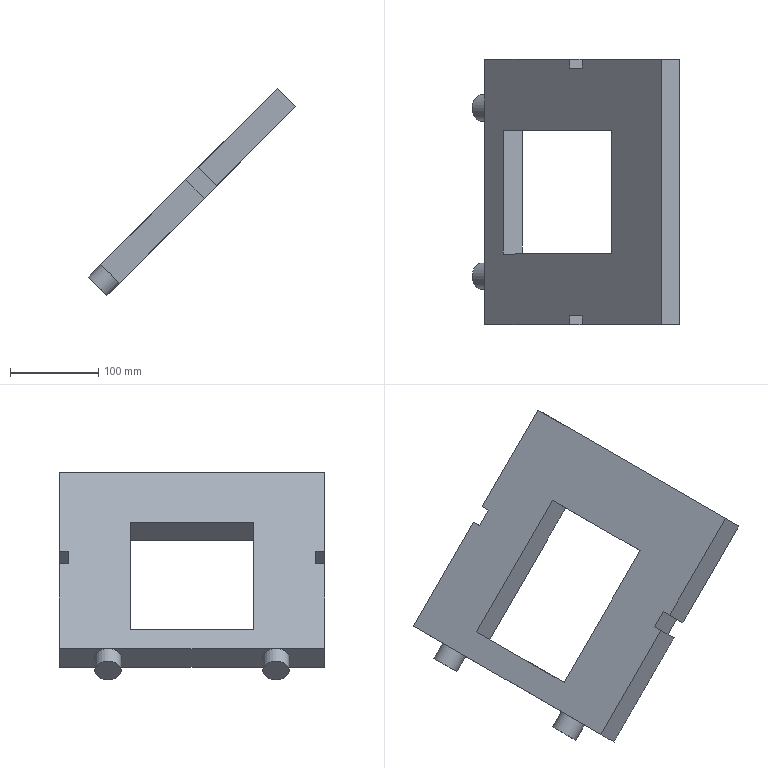Part | NX | features solid 2 | 1 solid | 24 faces | box 234.759 x 300 x 234.759 mm | volume 1831955 mm3 | plane 22 | cylinder 2 | commonest cylinder face diameters 30 x2
STEP:
#1=CARTESIAN_POINT('',(-1080.504,275.,-210.197));
#2=VERTEX_POINT('',#1);
#3=CARTESIAN_POINT('',(-1101.717,275.,-188.984));
#4=VERTEX_POINT('',#3);
#5=CARTESIAN_POINT('',(-1091.111,275.,-199.591));
#6=DIRECTION('',(-0.7071,0.,-0.7071));
#7=DIRECTION('',(0.7071,0.,-0.7071));
#8=AXIS2_PLACEMENT_3D('',#5,#6,#7);
#9=CIRCLE('',#8,15.);
#10=EDGE_CURVE('',#2,#4,#9,.T.);
#11=ORIENTED_EDGE('',*,*,#10,.F.);
#12=CARTESIAN_POINT('',(-1080.504,85.,-210.197));
#13=VERTEX_POINT('',#12);
#14=CARTESIAN_POINT('',(-1080.504,30.,-210.197));
#15=DIRECTION('',(0.,1.,0.));
#16=VECTOR('',#15,1000.);
#17=LINE('',#14,#16);
#18=EDGE_CURVE('',#13,#2,#17,.T.);
#19=ORIENTED_EDGE('',*,*,#18,.F.);
#20=CARTESIAN_POINT('',(-1101.717,85.,-188.984));
#21=VERTEX_POINT('',#20);
#22=CARTESIAN_POINT('',(-1091.111,85.,-199.591));
#23=DIRECTION('',(-0.7071,0.,-0.7071));
#24=DIRECTION('',(0.7071,0.,-0.7071));
#25=AXIS2_PLACEMENT_3D('',#22,#23,#24);
#26=CIRCLE('',#25,15.);
#27=EDGE_CURVE('',#21,#13,#26,.T.);
#28=ORIENTED_EDGE('',*,*,#27,.F.);
#29=CARTESIAN_POINT('',(-1101.717,30.,-188.984));
#30=DIRECTION('',(0.,1.,0.));
#31=VECTOR('',#30,1000.);
#32=LINE('',#29,#31);
#33=EDGE_CURVE('',#21,#4,#32,.T.);
#34=ORIENTED_EDGE('',*,*,#33,.T.);
#35=EDGE_LOOP('',(#11,#19,#28,#34));
#36=FACE_BOUND('',#35,.T.);
#37=CARTESIAN_POINT('',(-1080.504,30.,-210.197));
#38=DIRECTION('',(-0.7071,0.,-0.7071));
#39=DIRECTION('',(0.7071,0.,-0.7071));
#40=AXIS2_PLACEMENT_3D('',#37,#38,#39);
#41=PLANE('',#40);
#42=ADVANCED_FACE('',(#36),#41,.T.);
#43=CARTESIAN_POINT('',(-1091.111,85.,-199.591));
#44=DIRECTION('',(-0.7071,0.,-0.7071));
#45=DIRECTION('',(0.7071,0.,-0.7071));
#46=AXIS2_PLACEMENT_3D('',#43,#44,#45);
#47=CIRCLE('',#46,15.);
#48=EDGE_CURVE('',#13,#21,#47,.T.);
#49=ORIENTED_EDGE('',*,*,#48,.F.);
#50=CARTESIAN_POINT('',(-1080.504,30.,-210.197));
#51=VERTEX_POINT('',#50);
#52=CARTESIAN_POINT('',(-1080.504,30.,-210.197));
#53=DIRECTION('',(0.,1.,0.));
#54=VECTOR('',#53,1000.);
#55=LINE('',#52,#54);
#56=EDGE_CURVE('',#51,#13,#55,.T.);
#57=ORIENTED_EDGE('',*,*,#56,.F.);
#58=CARTESIAN_POINT('',(-1101.717,30.,-188.984));
#59=VERTEX_POINT('',#58);
#60=CARTESIAN_POINT('',(-1080.504,30.,-210.197));
#61=DIRECTION('',(-0.7071,0.,0.7071));
#62=VECTOR('',#61,1000.);
#63=LINE('',#60,#62);
#64=EDGE_CURVE('',#51,#59,#63,.T.);
#65=ORIENTED_EDGE('',*,*,#64,.T.);
#66=CARTESIAN_POINT('',(-1101.717,30.,-188.984));
#67=DIRECTION('',(0.,1.,0.));
#68=VECTOR('',#67,1000.);
#69=LINE('',#66,#68);
#70=EDGE_CURVE('',#59,#21,#69,.T.);
#71=ORIENTED_EDGE('',*,*,#70,.T.);
#72=EDGE_LOOP('',(#49,#57,#65,#71));
#73=FACE_BOUND('',#72,.T.);
#74=CARTESIAN_POINT('',(-1080.504,30.,-210.197));
#75=DIRECTION('',(-0.7071,0.,-0.7071));
#76=DIRECTION('',(0.7071,0.,-0.7071));
#77=AXIS2_PLACEMENT_3D('',#74,#75,#76);
#78=PLANE('',#77);
#79=ADVANCED_FACE('',(#73),#78,.T.);
#80=CARTESIAN_POINT('',(-991.665,30.,-78.932));
#81=VERTEX_POINT('',#80);
#82=CARTESIAN_POINT('',(-902.313,30.,10.42));
#83=VERTEX_POINT('',#82);
#84=CARTESIAN_POINT('',(-1137.073,30.,-224.34));
#85=DIRECTION('',(0.7071,0.,0.7071));
#86=VECTOR('',#85,1000.);
#87=LINE('',#84,#86);
#88=EDGE_CURVE('',#81,#83,#87,.T.);
#89=ORIENTED_EDGE('',*,*,#88,.F.);
#90=CARTESIAN_POINT('',(-970.452,30.,-100.145));
#91=VERTEX_POINT('',#90);
#92=CARTESIAN_POINT('',(-1023.864,30.,-46.733));
#93=DIRECTION('',(-0.7071,0.,0.7071));
#94=VECTOR('',#93,1000.);
#95=LINE('',#92,#94);
#96=EDGE_CURVE('',#91,#81,#95,.T.);
#97=ORIENTED_EDGE('',*,*,#96,.F.);
#98=CARTESIAN_POINT('',(-881.1,30.,-10.793));
#99=VERTEX_POINT('',#98);
#100=CARTESIAN_POINT('',(-916.455,30.,-46.149));
#101=DIRECTION('',(-0.7071,0.,-0.7071));
#102=VECTOR('',#101,1000.);
#103=LINE('',#100,#102);
#104=EDGE_CURVE('',#99,#91,#103,.T.);
#105=ORIENTED_EDGE('',*,*,#104,.F.);
#106=CARTESIAN_POINT('',(-902.313,30.,10.42));
#107=DIRECTION('',(0.7071,0.,-0.7071));
#108=VECTOR('',#107,1000.);
#109=LINE('',#106,#108);
#110=EDGE_CURVE('',#83,#99,#109,.T.);
#111=ORIENTED_EDGE('',*,*,#110,.F.);
#112=EDGE_LOOP('',(#89,#97,#105,#111));
#113=FACE_BOUND('',#112,.T.);
#114=CARTESIAN_POINT('',(-1137.073,30.,-224.34));
#115=DIRECTION('',(0.,-1.,0.));
#116=DIRECTION('',(0.9963,0.,0.08598));
#117=AXIS2_PLACEMENT_3D('',#114,#115,#116);
#118=PLANE('',#117);
#119=ADVANCED_FACE('',(#113),#118,.T.);
#120=CARTESIAN_POINT('',(-958.882,250.,-46.149));
#121=VERTEX_POINT('',#120);
#122=CARTESIAN_POINT('',(-958.882,110.,-46.149));
#123=VERTEX_POINT('',#122);
#124=CARTESIAN_POINT('',(-958.882,250.,-46.149));
#125=DIRECTION('',(0.,-1.,0.));
#126=VECTOR('',#125,1000.);
#127=LINE('',#124,#126);
#128=EDGE_CURVE('',#121,#123,#127,.T.);
#129=ORIENTED_EDGE('',*,*,#128,.T.);
#130=CARTESIAN_POINT('',(-1080.504,110.,-167.771));
#131=VERTEX_POINT('',#130);
#132=CARTESIAN_POINT('',(-1137.073,110.,-224.34));
#133=DIRECTION('',(0.7071,0.,0.7071));
#134=VECTOR('',#133,1000.);
#135=LINE('',#132,#134);
#136=EDGE_CURVE('',#131,#123,#135,.T.);
#137=ORIENTED_EDGE('',*,*,#136,.F.);
#138=CARTESIAN_POINT('',(-1080.504,250.,-167.771));
#139=VERTEX_POINT('',#138);
#140=CARTESIAN_POINT('',(-1080.504,250.,-167.771));
#141=DIRECTION('',(0.,-1.,0.));
#142=VECTOR('',#141,1000.);
#143=LINE('',#140,#142);
#144=EDGE_CURVE('',#139,#131,#143,.T.);
#145=ORIENTED_EDGE('',*,*,#144,.F.);
#146=CARTESIAN_POINT('',(-1137.073,250.,-224.34));
#147=DIRECTION('',(0.7071,0.,0.7071));
#148=VECTOR('',#147,1000.);
#149=LINE('',#146,#148);
#150=EDGE_CURVE('',#139,#121,#149,.T.);
#151=ORIENTED_EDGE('',*,*,#150,.T.);
#152=EDGE_LOOP('',(#129,#137,#145,#151));
#153=FACE_BOUND('',#152,.T.);
#154=CARTESIAN_POINT('',(-1005.712,30.,-92.979));
#155=VERTEX_POINT('',#154);
#156=CARTESIAN_POINT('',(-1005.712,40.,-92.979));
#157=VERTEX_POINT('',#156);
#158=CARTESIAN_POINT('',(-1005.712,40.,-92.979));
#159=DIRECTION('',(0.,1.,0.));
#160=VECTOR('',#159,1000.);
#161=LINE('',#158,#160);
#162=EDGE_CURVE('',#155,#157,#161,.T.);
#163=ORIENTED_EDGE('',*,*,#162,.T.);
#164=CARTESIAN_POINT('',(-991.665,40.,-78.932));
#165=VERTEX_POINT('',#164);
#166=CARTESIAN_POINT('',(-1137.073,40.,-224.34));
#167=DIRECTION('',(0.7071,0.,0.7071));
#168=VECTOR('',#167,1000.);
#169=LINE('',#166,#168);
#170=EDGE_CURVE('',#165,#157,#169,.F.);
#171=ORIENTED_EDGE('',*,*,#170,.F.);
#172=CARTESIAN_POINT('',(-991.665,40.,-78.932));
#173=DIRECTION('',(0.,1.,0.));
#174=VECTOR('',#173,1000.);
#175=LINE('',#172,#174);
#176=EDGE_CURVE('',#81,#165,#175,.T.);
#177=ORIENTED_EDGE('',*,*,#176,.F.);
#178=ORIENTED_EDGE('',*,*,#88,.T.);
#179=CARTESIAN_POINT('',(-902.313,330.,10.42));
#180=VERTEX_POINT('',#179);
#181=CARTESIAN_POINT('',(-902.313,30.,10.42));
#182=DIRECTION('',(0.,1.,0.));
#183=VECTOR('',#182,1000.);
#184=LINE('',#181,#183);
#185=EDGE_CURVE('',#83,#180,#184,.T.);
#186=ORIENTED_EDGE('',*,*,#185,.T.);
#187=CARTESIAN_POINT('',(-991.665,330.,-78.932));
#188=VERTEX_POINT('',#187);
#189=CARTESIAN_POINT('',(-1137.073,330.,-224.34));
#190=DIRECTION('',(0.7071,0.,0.7071));
#191=VECTOR('',#190,1000.);
#192=LINE('',#189,#191);
#193=EDGE_CURVE('',#188,#180,#192,.T.);
#194=ORIENTED_EDGE('',*,*,#193,.F.);
#195=CARTESIAN_POINT('',(-991.665,320.,-78.932));
#196=VERTEX_POINT('',#195);
#197=CARTESIAN_POINT('',(-991.665,320.,-78.932));
#198=DIRECTION('',(0.,1.,0.));
#199=VECTOR('',#198,1000.);
#200=LINE('',#197,#199);
#201=EDGE_CURVE('',#188,#196,#200,.F.);
#202=ORIENTED_EDGE('',*,*,#201,.T.);
#203=CARTESIAN_POINT('',(-1005.712,320.,-92.979));
#204=VERTEX_POINT('',#203);
#205=CARTESIAN_POINT('',(-1137.073,320.,-224.34));
#206=DIRECTION('',(0.7071,0.,0.7071));
#207=VECTOR('',#206,1000.);
#208=LINE('',#205,#207);
#209=EDGE_CURVE('',#196,#204,#208,.F.);
#210=ORIENTED_EDGE('',*,*,#209,.T.);
#211=CARTESIAN_POINT('',(-1005.712,330.,-92.979));
#212=VERTEX_POINT('',#211);
#213=CARTESIAN_POINT('',(-1005.712,320.,-92.979));
#214=DIRECTION('',(0.,1.,0.));
#215=VECTOR('',#214,1000.);
#216=LINE('',#213,#215);
#217=EDGE_CURVE('',#212,#204,#216,.F.);
#218=ORIENTED_EDGE('',*,*,#217,.F.);
#219=CARTESIAN_POINT('',(-1101.717,330.,-188.984));
#220=VERTEX_POINT('',#219);
#221=CARTESIAN_POINT('',(-1137.073,330.,-224.34));
#222=DIRECTION('',(0.7071,0.,0.7071));
#223=VECTOR('',#222,1000.);
#224=LINE('',#221,#223);
#225=EDGE_CURVE('',#220,#212,#224,.T.);
#226=ORIENTED_EDGE('',*,*,#225,.F.);
#227=CARTESIAN_POINT('',(-1101.717,30.,-188.984));
#228=DIRECTION('',(0.,1.,0.));
#229=VECTOR('',#228,1000.);
#230=LINE('',#227,#229);
#231=EDGE_CURVE('',#4,#220,#230,.T.);
#232=ORIENTED_EDGE('',*,*,#231,.F.);
#233=ORIENTED_EDGE('',*,*,#33,.F.);
#234=ORIENTED_EDGE('',*,*,#70,.F.);
#235=CARTESIAN_POINT('',(-1137.073,30.,-224.34));
#236=DIRECTION('',(0.7071,0.,0.7071));
#237=VECTOR('',#236,1000.);
#238=LINE('',#235,#237);
#239=EDGE_CURVE('',#59,#155,#238,.T.);
#240=ORIENTED_EDGE('',*,*,#239,.T.);
#241=EDGE_LOOP('',(#163,#171,#177,#178,#186,#194,#202,#210,#218,#226,#232,#233,#234,#240));
#242=FACE_BOUND('',#241,.T.);
#243=CARTESIAN_POINT('',(-1137.073,30.,-224.34));
#244=DIRECTION('',(-0.7071,0.,0.7071));
#245=DIRECTION('',(-0.7071,0.,-0.7071));
#246=AXIS2_PLACEMENT_3D('',#243,#244,#245);
#247=PLANE('',#246);
#248=ADVANCED_FACE('',(#153,#242),#247,.T.);
#249=CARTESIAN_POINT('',(-881.1,330.,-10.793));
#250=VERTEX_POINT('',#249);
#251=CARTESIAN_POINT('',(-881.1,30.,-10.793));
#252=DIRECTION('',(0.,1.,0.));
#253=VECTOR('',#252,1000.);
#254=LINE('',#251,#253);
#255=EDGE_CURVE('',#99,#250,#254,.T.);
#256=ORIENTED_EDGE('',*,*,#255,.T.);
#257=CARTESIAN_POINT('',(-902.313,330.,10.42));
#258=DIRECTION('',(0.7071,0.,-0.7071));
#259=VECTOR('',#258,1000.);
#260=LINE('',#257,#259);
#261=EDGE_CURVE('',#180,#250,#260,.T.);
#262=ORIENTED_EDGE('',*,*,#261,.F.);
#263=ORIENTED_EDGE('',*,*,#185,.F.);
#264=ORIENTED_EDGE('',*,*,#110,.T.);
#265=EDGE_LOOP('',(#256,#262,#263,#264));
#266=FACE_BOUND('',#265,.T.);
#267=CARTESIAN_POINT('',(-902.313,30.,10.42));
#268=DIRECTION('',(0.7071,0.,0.7071));
#269=DIRECTION('',(-0.7071,0.,0.7071));
#270=AXIS2_PLACEMENT_3D('',#267,#268,#269);
#271=PLANE('',#270);
#272=ADVANCED_FACE('',(#266),#271,.T.);
#273=CARTESIAN_POINT('',(-1059.291,250.,-188.984));
#274=VERTEX_POINT('',#273);
#275=CARTESIAN_POINT('',(-1059.291,110.,-188.984));
#276=VERTEX_POINT('',#275);
#277=CARTESIAN_POINT('',(-1059.291,250.,-188.984));
#278=DIRECTION('',(0.,-1.,0.));
#279=VECTOR('',#278,1000.);
#280=LINE('',#277,#279);
#281=EDGE_CURVE('',#274,#276,#280,.T.);
#282=ORIENTED_EDGE('',*,*,#281,.T.);
#283=CARTESIAN_POINT('',(-937.669,110.,-67.362));
#284=VERTEX_POINT('',#283);
#285=CARTESIAN_POINT('',(-916.455,110.,-46.149));
#286=DIRECTION('',(-0.7071,0.,-0.7071));
#287=VECTOR('',#286,1000.);
#288=LINE('',#285,#287);
#289=EDGE_CURVE('',#284,#276,#288,.T.);
#290=ORIENTED_EDGE('',*,*,#289,.F.);
#291=CARTESIAN_POINT('',(-937.669,250.,-67.362));
#292=VERTEX_POINT('',#291);
#293=CARTESIAN_POINT('',(-937.669,250.,-67.362));
#294=DIRECTION('',(0.,-1.,0.));
#295=VECTOR('',#294,1000.);
#296=LINE('',#293,#295);
#297=EDGE_CURVE('',#292,#284,#296,.T.);
#298=ORIENTED_EDGE('',*,*,#297,.F.);
#299=CARTESIAN_POINT('',(-916.455,250.,-46.149));
#300=DIRECTION('',(-0.7071,0.,-0.7071));
#301=VECTOR('',#300,1000.);
#302=LINE('',#299,#301);
#303=EDGE_CURVE('',#292,#274,#302,.T.);
#304=ORIENTED_EDGE('',*,*,#303,.T.);
#305=EDGE_LOOP('',(#282,#290,#298,#304));
#306=FACE_BOUND('',#305,.T.);
#307=CARTESIAN_POINT('',(-984.499,30.,-114.192));
#308=VERTEX_POINT('',#307);
#309=CARTESIAN_POINT('',(-984.499,40.,-114.192));
#310=VERTEX_POINT('',#309);
#311=CARTESIAN_POINT('',(-984.499,30.,-114.192));
#312=DIRECTION('',(0.,1.,0.));
#313=VECTOR('',#312,1000.);
#314=LINE('',#311,#313);
#315=EDGE_CURVE('',#308,#310,#314,.T.);
#316=ORIENTED_EDGE('',*,*,#315,.F.);
#317=CARTESIAN_POINT('',(-916.455,30.,-46.149));
#318=DIRECTION('',(-0.7071,0.,-0.7071));
#319=VECTOR('',#318,1000.);
#320=LINE('',#317,#319);
#321=EDGE_CURVE('',#308,#51,#320,.T.);
#322=ORIENTED_EDGE('',*,*,#321,.T.);
#323=ORIENTED_EDGE('',*,*,#56,.T.);
#324=ORIENTED_EDGE('',*,*,#18,.T.);
#325=CARTESIAN_POINT('',(-1080.504,330.,-210.197));
#326=VERTEX_POINT('',#325);
#327=CARTESIAN_POINT('',(-1080.504,30.,-210.197));
#328=DIRECTION('',(0.,1.,0.));
#329=VECTOR('',#328,1000.);
#330=LINE('',#327,#329);
#331=EDGE_CURVE('',#2,#326,#330,.T.);
#332=ORIENTED_EDGE('',*,*,#331,.T.);
#333=CARTESIAN_POINT('',(-984.499,330.,-114.192));
#334=VERTEX_POINT('',#333);
#335=CARTESIAN_POINT('',(-916.455,330.,-46.149));
#336=DIRECTION('',(-0.7071,0.,-0.7071));
#337=VECTOR('',#336,1000.);
#338=LINE('',#335,#337);
#339=EDGE_CURVE('',#334,#326,#338,.T.);
#340=ORIENTED_EDGE('',*,*,#339,.F.);
#341=CARTESIAN_POINT('',(-984.499,320.,-114.192));
#342=VERTEX_POINT('',#341);
#343=CARTESIAN_POINT('',(-984.499,30.,-114.192));
#344=DIRECTION('',(0.,1.,0.));
#345=VECTOR('',#344,1000.);
#346=LINE('',#343,#345);
#347=EDGE_CURVE('',#334,#342,#346,.F.);
#348=ORIENTED_EDGE('',*,*,#347,.T.);
#349=CARTESIAN_POINT('',(-970.452,320.,-100.145));
#350=VERTEX_POINT('',#349);
#351=CARTESIAN_POINT('',(-1115.86,320.,-245.553));
#352=DIRECTION('',(0.7071,0.,0.7071));
#353=VECTOR('',#352,1000.);
#354=LINE('',#351,#353);
#355=EDGE_CURVE('',#350,#342,#354,.F.);
#356=ORIENTED_EDGE('',*,*,#355,.F.);
#357=CARTESIAN_POINT('',(-970.452,330.,-100.145));
#358=VERTEX_POINT('',#357);
#359=CARTESIAN_POINT('',(-970.452,30.,-100.145));
#360=DIRECTION('',(0.,1.,0.));
#361=VECTOR('',#360,1000.);
#362=LINE('',#359,#361);
#363=EDGE_CURVE('',#358,#350,#362,.F.);
#364=ORIENTED_EDGE('',*,*,#363,.F.);
#365=CARTESIAN_POINT('',(-916.455,330.,-46.149));
#366=DIRECTION('',(-0.7071,0.,-0.7071));
#367=VECTOR('',#366,1000.);
#368=LINE('',#365,#367);
#369=EDGE_CURVE('',#250,#358,#368,.T.);
#370=ORIENTED_EDGE('',*,*,#369,.F.);
#371=ORIENTED_EDGE('',*,*,#255,.F.);
#372=ORIENTED_EDGE('',*,*,#104,.T.);
#373=CARTESIAN_POINT('',(-970.452,40.,-100.145));
#374=VERTEX_POINT('',#373);
#375=CARTESIAN_POINT('',(-970.452,30.,-100.145));
#376=DIRECTION('',(0.,1.,0.));
#377=VECTOR('',#376,1000.);
#378=LINE('',#375,#377);
#379=EDGE_CURVE('',#91,#374,#378,.T.);
#380=ORIENTED_EDGE('',*,*,#379,.T.);
#381=CARTESIAN_POINT('',(-1115.86,40.,-245.553));
#382=DIRECTION('',(0.7071,0.,0.7071));
#383=VECTOR('',#382,1000.);
#384=LINE('',#381,#383);
#385=EDGE_CURVE('',#374,#310,#384,.F.);
#386=ORIENTED_EDGE('',*,*,#385,.T.);
#387=EDGE_LOOP('',(#316,#322,#323,#324,#332,#340,#348,#356,#364,#370,#371,#372,#380,#386));
#388=FACE_BOUND('',#387,.T.);
#389=CARTESIAN_POINT('',(-916.455,30.,-46.149));
#390=DIRECTION('',(0.7071,0.,-0.7071));
#391=DIRECTION('',(0.7071,0.,0.7071));
#392=AXIS2_PLACEMENT_3D('',#389,#390,#391);
#393=PLANE('',#392);
#394=ADVANCED_FACE('',(#306,#388),#393,.T.);
#395=CARTESIAN_POINT('',(-1091.111,275.,-199.591));
#396=DIRECTION('',(0.7071,0.,0.7071));
#397=DIRECTION('',(0.7071,0.,-0.7071));
#398=AXIS2_PLACEMENT_3D('',#395,#396,#397);
#399=CIRCLE('',#398,15.);
#400=EDGE_CURVE('',#2,#4,#399,.T.);
#401=ORIENTED_EDGE('',*,*,#400,.T.);
#402=ORIENTED_EDGE('',*,*,#231,.T.);
#403=CARTESIAN_POINT('',(-1080.504,330.,-210.197));
#404=DIRECTION('',(-0.7071,0.,0.7071));
#405=VECTOR('',#404,1000.);
#406=LINE('',#403,#405);
#407=EDGE_CURVE('',#326,#220,#406,.T.);
#408=ORIENTED_EDGE('',*,*,#407,.F.);
#409=ORIENTED_EDGE('',*,*,#331,.F.);
#410=EDGE_LOOP('',(#401,#402,#408,#409));
#411=FACE_BOUND('',#410,.T.);
#412=CARTESIAN_POINT('',(-1080.504,30.,-210.197));
#413=DIRECTION('',(-0.7071,0.,-0.7071));
#414=DIRECTION('',(0.7071,0.,-0.7071));
#415=AXIS2_PLACEMENT_3D('',#412,#413,#414);
#416=PLANE('',#415);
#417=ADVANCED_FACE('',(#411),#416,.T.);
#418=CARTESIAN_POINT('',(-1036.273,30.,-62.418));
#419=DIRECTION('',(-0.7071,0.,0.7071));
#420=VECTOR('',#419,1000.);
#421=LINE('',#418,#420);
#422=EDGE_CURVE('',#308,#155,#421,.T.);
#423=ORIENTED_EDGE('',*,*,#422,.T.);
#424=ORIENTED_EDGE('',*,*,#239,.F.);
#425=ORIENTED_EDGE('',*,*,#64,.F.);
#426=ORIENTED_EDGE('',*,*,#321,.F.);
#427=EDGE_LOOP('',(#423,#424,#425,#426));
#428=FACE_BOUND('',#427,.T.);
#429=CARTESIAN_POINT('',(-1137.073,30.,-224.34));
#430=DIRECTION('',(0.,-1.,0.));
#431=DIRECTION('',(0.9963,0.,0.08598));
#432=AXIS2_PLACEMENT_3D('',#429,#430,#431);
#433=PLANE('',#432);
#434=ADVANCED_FACE('',(#428),#433,.T.);
#435=ORIENTED_EDGE('',*,*,#289,.T.);
#436=CARTESIAN_POINT('',(-1059.291,110.,-188.984));
#437=DIRECTION('',(-0.7071,0.,0.7071));
#438=VECTOR('',#437,1000.);
#439=LINE('',#436,#438);
#440=EDGE_CURVE('',#276,#131,#439,.T.);
#441=ORIENTED_EDGE('',*,*,#440,.T.);
#442=ORIENTED_EDGE('',*,*,#136,.T.);
#443=CARTESIAN_POINT('',(-958.882,110.,-46.149));
#444=DIRECTION('',(0.7071,0.,-0.7071));
#445=VECTOR('',#444,1000.);
#446=LINE('',#443,#445);
#447=EDGE_CURVE('',#123,#284,#446,.T.);
#448=ORIENTED_EDGE('',*,*,#447,.T.);
#449=EDGE_LOOP('',(#435,#441,#442,#448));
#450=FACE_BOUND('',#449,.T.);
#451=CARTESIAN_POINT('',(-1137.073,110.,-224.34));
#452=DIRECTION('',(0.,-1.,0.));
#453=DIRECTION('',(0.9963,0.,0.08598));
#454=AXIS2_PLACEMENT_3D('',#451,#452,#453);
#455=PLANE('',#454);
#456=ADVANCED_FACE('',(#450),#455,.F.);
#457=ORIENTED_EDGE('',*,*,#385,.F.);
#458=CARTESIAN_POINT('',(-1023.864,40.,-46.733));
#459=DIRECTION('',(-0.7071,0.,0.7071));
#460=VECTOR('',#459,1000.);
#461=LINE('',#458,#460);
#462=EDGE_CURVE('',#374,#165,#461,.T.);
#463=ORIENTED_EDGE('',*,*,#462,.T.);
#464=ORIENTED_EDGE('',*,*,#170,.T.);
#465=CARTESIAN_POINT('',(-1036.273,40.,-62.418));
#466=DIRECTION('',(-0.7071,0.,0.7071));
#467=VECTOR('',#466,1000.);
#468=LINE('',#465,#467);
#469=EDGE_CURVE('',#310,#157,#468,.T.);
#470=ORIENTED_EDGE('',*,*,#469,.F.);
#471=EDGE_LOOP('',(#457,#463,#464,#470));
#472=FACE_BOUND('',#471,.T.);
#473=CARTESIAN_POINT('',(-1115.86,40.,-245.553));
#474=DIRECTION('',(0.,-1.,0.));
#475=DIRECTION('',(-0.7071,0.,0.7071));
#476=AXIS2_PLACEMENT_3D('',#473,#474,#475);
#477=PLANE('',#476);
#478=ADVANCED_FACE('',(#472),#477,.T.);
#479=ORIENTED_EDGE('',*,*,#469,.T.);
#480=ORIENTED_EDGE('',*,*,#162,.F.);
#481=ORIENTED_EDGE('',*,*,#422,.F.);
#482=ORIENTED_EDGE('',*,*,#315,.T.);
#483=EDGE_LOOP('',(#479,#480,#481,#482));
#484=FACE_BOUND('',#483,.T.);
#485=CARTESIAN_POINT('',(-1036.273,40.,-62.418));
#486=DIRECTION('',(-0.7071,0.,-0.7071));
#487=DIRECTION('',(0.7071,0.,-0.7071));
#488=AXIS2_PLACEMENT_3D('',#485,#486,#487);
#489=PLANE('',#488);
#490=ADVANCED_FACE('',(#484),#489,.F.);
#491=ORIENTED_EDGE('',*,*,#462,.F.);
#492=ORIENTED_EDGE('',*,*,#379,.F.);
#493=ORIENTED_EDGE('',*,*,#96,.T.);
#494=ORIENTED_EDGE('',*,*,#176,.T.);
#495=EDGE_LOOP('',(#491,#492,#493,#494));
#496=FACE_BOUND('',#495,.T.);
#497=CARTESIAN_POINT('',(-1023.864,40.,-46.733));
#498=DIRECTION('',(-0.7071,0.,-0.7071));
#499=DIRECTION('',(0.7071,0.,-0.7071));
#500=AXIS2_PLACEMENT_3D('',#497,#498,#499);
#501=PLANE('',#500);
#502=ADVANCED_FACE('',(#496),#501,.T.);
#503=ORIENTED_EDGE('',*,*,#303,.F.);
#504=CARTESIAN_POINT('',(-958.882,250.,-46.149));
#505=DIRECTION('',(0.7071,0.,-0.7071));
#506=VECTOR('',#505,1000.);
#507=LINE('',#504,#506);
#508=EDGE_CURVE('',#121,#292,#507,.T.);
#509=ORIENTED_EDGE('',*,*,#508,.F.);
#510=ORIENTED_EDGE('',*,*,#150,.F.);
#511=CARTESIAN_POINT('',(-1059.291,250.,-188.984));
#512=DIRECTION('',(-0.7071,0.,0.7071));
#513=VECTOR('',#512,1000.);
#514=LINE('',#511,#513);
#515=EDGE_CURVE('',#274,#139,#514,.T.);
#516=ORIENTED_EDGE('',*,*,#515,.F.);
#517=EDGE_LOOP('',(#503,#509,#510,#516));
#518=FACE_BOUND('',#517,.T.);
#519=CARTESIAN_POINT('',(-1137.073,250.,-224.34));
#520=DIRECTION('',(0.,1.,0.));
#521=DIRECTION('',(0.9963,0.,0.08598));
#522=AXIS2_PLACEMENT_3D('',#519,#520,#521);
#523=PLANE('',#522);
#524=ADVANCED_FACE('',(#518),#523,.F.);
#525=ORIENTED_EDGE('',*,*,#225,.T.);
#526=CARTESIAN_POINT('',(-1036.273,330.,-62.418));
#527=DIRECTION('',(0.7071,0.,-0.7071));
#528=VECTOR('',#527,1000.);
#529=LINE('',#526,#528);
#530=EDGE_CURVE('',#334,#212,#529,.F.);
#531=ORIENTED_EDGE('',*,*,#530,.F.);
#532=ORIENTED_EDGE('',*,*,#339,.T.);
#533=ORIENTED_EDGE('',*,*,#407,.T.);
#534=EDGE_LOOP('',(#525,#531,#532,#533));
#535=FACE_BOUND('',#534,.T.);
#536=CARTESIAN_POINT('',(-1137.073,330.,-224.34));
#537=DIRECTION('',(0.,1.,0.));
#538=DIRECTION('',(0.9963,0.,0.08598));
#539=AXIS2_PLACEMENT_3D('',#536,#537,#538);
#540=PLANE('',#539);
#541=ADVANCED_FACE('',(#535),#540,.T.);
#542=CARTESIAN_POINT('',(-1023.864,330.,-46.733));
#543=DIRECTION('',(0.7071,0.,-0.7071));
#544=VECTOR('',#543,1000.);
#545=LINE('',#542,#544);
#546=EDGE_CURVE('',#358,#188,#545,.F.);
#547=ORIENTED_EDGE('',*,*,#546,.T.);
#548=ORIENTED_EDGE('',*,*,#193,.T.);
#549=ORIENTED_EDGE('',*,*,#261,.T.);
#550=ORIENTED_EDGE('',*,*,#369,.T.);
#551=EDGE_LOOP('',(#547,#548,#549,#550));
#552=FACE_BOUND('',#551,.T.);
#553=CARTESIAN_POINT('',(-1137.073,330.,-224.34));
#554=DIRECTION('',(0.,1.,0.));
#555=DIRECTION('',(0.9963,0.,0.08598));
#556=AXIS2_PLACEMENT_3D('',#553,#554,#555);
#557=PLANE('',#556);
#558=ADVANCED_FACE('',(#552),#557,.T.);
#559=ORIENTED_EDGE('',*,*,#209,.F.);
#560=CARTESIAN_POINT('',(-1023.864,320.,-46.733));
#561=DIRECTION('',(0.7071,0.,-0.7071));
#562=VECTOR('',#561,1000.);
#563=LINE('',#560,#562);
#564=EDGE_CURVE('',#350,#196,#563,.F.);
#565=ORIENTED_EDGE('',*,*,#564,.F.);
#566=ORIENTED_EDGE('',*,*,#355,.T.);
#567=CARTESIAN_POINT('',(-1036.273,320.,-62.418));
#568=DIRECTION('',(0.7071,0.,-0.7071));
#569=VECTOR('',#568,1000.);
#570=LINE('',#567,#569);
#571=EDGE_CURVE('',#342,#204,#570,.F.);
#572=ORIENTED_EDGE('',*,*,#571,.T.);
#573=EDGE_LOOP('',(#559,#565,#566,#572));
#574=FACE_BOUND('',#573,.T.);
#575=CARTESIAN_POINT('',(-1115.86,320.,-245.553));
#576=DIRECTION('',(0.,1.,0.));
#577=DIRECTION('',(-0.7071,0.,0.7071));
#578=AXIS2_PLACEMENT_3D('',#575,#576,#577);
#579=PLANE('',#578);
#580=ADVANCED_FACE('',(#574),#579,.T.);
#581=ORIENTED_EDGE('',*,*,#571,.F.);
#582=ORIENTED_EDGE('',*,*,#347,.F.);
#583=ORIENTED_EDGE('',*,*,#530,.T.);
#584=ORIENTED_EDGE('',*,*,#217,.T.);
#585=EDGE_LOOP('',(#581,#582,#583,#584));
#586=FACE_BOUND('',#585,.T.);
#587=CARTESIAN_POINT('',(-1036.273,320.,-62.418));
#588=DIRECTION('',(-0.7071,0.,-0.7071));
#589=DIRECTION('',(0.7071,0.,-0.7071));
#590=AXIS2_PLACEMENT_3D('',#587,#588,#589);
#591=PLANE('',#590);
#592=ADVANCED_FACE('',(#586),#591,.F.);
#593=ORIENTED_EDGE('',*,*,#564,.T.);
#594=ORIENTED_EDGE('',*,*,#201,.F.);
#595=ORIENTED_EDGE('',*,*,#546,.F.);
#596=ORIENTED_EDGE('',*,*,#363,.T.);
#597=EDGE_LOOP('',(#593,#594,#595,#596));
#598=FACE_BOUND('',#597,.T.);
#599=CARTESIAN_POINT('',(-1023.864,320.,-46.733));
#600=DIRECTION('',(-0.7071,0.,-0.7071));
#601=DIRECTION('',(0.7071,0.,-0.7071));
#602=AXIS2_PLACEMENT_3D('',#599,#600,#601);
#603=PLANE('',#602);
#604=ADVANCED_FACE('',(#598),#603,.T.);
#605=ORIENTED_EDGE('',*,*,#440,.F.);
#606=ORIENTED_EDGE('',*,*,#281,.F.);
#607=ORIENTED_EDGE('',*,*,#515,.T.);
#608=ORIENTED_EDGE('',*,*,#144,.T.);
#609=EDGE_LOOP('',(#605,#606,#607,#608));
#610=FACE_BOUND('',#609,.T.);
#611=CARTESIAN_POINT('',(-1059.291,250.,-188.984));
#612=DIRECTION('',(0.7071,0.,0.7071));
#613=DIRECTION('',(-0.7071,0.,0.7071));
#614=AXIS2_PLACEMENT_3D('',#611,#612,#613);
#615=PLANE('',#614);
#616=ADVANCED_FACE('',(#610),#615,.T.);
#617=ORIENTED_EDGE('',*,*,#447,.F.);
#618=ORIENTED_EDGE('',*,*,#128,.F.);
#619=ORIENTED_EDGE('',*,*,#508,.T.);
#620=ORIENTED_EDGE('',*,*,#297,.T.);
#621=EDGE_LOOP('',(#617,#618,#619,#620));
#622=FACE_BOUND('',#621,.T.);
#623=CARTESIAN_POINT('',(-958.882,250.,-46.149));
#624=DIRECTION('',(-0.7071,0.,-0.7071));
#625=DIRECTION('',(0.7071,0.,-0.7071));
#626=AXIS2_PLACEMENT_3D('',#623,#624,#625);
#627=PLANE('',#626);
#628=ADVANCED_FACE('',(#622),#627,.T.);
#629=CARTESIAN_POINT('',(-1094.646,85.,-224.34));
#630=VERTEX_POINT('',#629);
#631=CARTESIAN_POINT('',(-1105.253,85.,-213.733));
#632=DIRECTION('',(-0.7071,0.,-0.7071));
#633=DIRECTION('',(0.7071,0.,-0.7071));
#634=AXIS2_PLACEMENT_3D('',#631,#632,#633);
#635=CIRCLE('',#634,15.);
#636=EDGE_CURVE('',#630,#630,#635,.T.);
#637=ORIENTED_EDGE('',*,*,#636,.T.);
#638=EDGE_LOOP('',(#637));
#639=FACE_BOUND('',#638,.T.);
#640=CARTESIAN_POINT('',(-1105.253,85.,-213.733));
#641=DIRECTION('',(-0.7071,0.,-0.7071));
#642=DIRECTION('',(0.7071,0.,-0.7071));
#643=AXIS2_PLACEMENT_3D('',#640,#641,#642);
#644=PLANE('',#643);
#645=ADVANCED_FACE('',(#639),#644,.T.);
#646=ORIENTED_EDGE('',*,*,#636,.F.);
#647=EDGE_LOOP('',(#646));
#648=FACE_BOUND('',#647,.T.);
#649=ORIENTED_EDGE('',*,*,#48,.T.);
#650=ORIENTED_EDGE('',*,*,#27,.T.);
#651=EDGE_LOOP('',(#649,#650));
#652=FACE_BOUND('',#651,.T.);
#653=CARTESIAN_POINT('',(-1126.466,85.,-234.946));
#654=DIRECTION('',(-0.7071,0.,-0.7071));
#655=DIRECTION('',(0.7071,0.,-0.7071));
#656=AXIS2_PLACEMENT_3D('',#653,#654,#655);
#657=CYLINDRICAL_SURFACE('',#656,15.);
#658=ADVANCED_FACE('',(#648,#652),#657,.T.);
#659=CARTESIAN_POINT('',(-1094.646,275.,-224.34));
#660=VERTEX_POINT('',#659);
#661=CARTESIAN_POINT('',(-1105.253,275.,-213.733));
#662=DIRECTION('',(0.7071,0.,0.7071));
#663=DIRECTION('',(0.7071,0.,-0.7071));
#664=AXIS2_PLACEMENT_3D('',#661,#662,#663);
#665=CIRCLE('',#664,15.);
#666=EDGE_CURVE('',#660,#660,#665,.T.);
#667=ORIENTED_EDGE('',*,*,#666,.F.);
#668=EDGE_LOOP('',(#667));
#669=FACE_BOUND('',#668,.T.);
#670=CARTESIAN_POINT('',(-1105.253,275.,-213.733));
#671=DIRECTION('',(-0.7071,0.,-0.7071));
#672=DIRECTION('',(0.7071,0.,-0.7071));
#673=AXIS2_PLACEMENT_3D('',#670,#671,#672);
#674=PLANE('',#673);
#675=ADVANCED_FACE('',(#669),#674,.T.);
#676=ORIENTED_EDGE('',*,*,#666,.T.);
#677=EDGE_LOOP('',(#676));
#678=FACE_BOUND('',#677,.T.);
#679=ORIENTED_EDGE('',*,*,#400,.F.);
#680=ORIENTED_EDGE('',*,*,#10,.T.);
#681=EDGE_LOOP('',(#679,#680));
#682=FACE_BOUND('',#681,.T.);
#683=CARTESIAN_POINT('',(-1126.466,275.,-234.946));
#684=DIRECTION('',(-0.7071,0.,-0.7071));
#685=DIRECTION('',(0.7071,0.,-0.7071));
#686=AXIS2_PLACEMENT_3D('',#683,#684,#685);
#687=CYLINDRICAL_SURFACE('',#686,15.);
#688=ADVANCED_FACE('',(#678,#682),#687,.T.);
#689=CLOSED_SHELL('',(#42,#79,#119,#248,#272,#394,#417,#434,#456,#478,#490,#502,#524,#541,#558,#580,#592,#604,#616,#628,#645,#658,#675,#688));
#690=MANIFOLD_SOLID_BREP('',#689);
#691=(LENGTH_UNIT()NAMED_UNIT(*)SI_UNIT(.MILLI.,.METRE.));
#692=UNCERTAINTY_MEASURE_WITH_UNIT(LENGTH_MEASURE(0.00001),#691,'','');
#693=(NAMED_UNIT(*)PLANE_ANGLE_UNIT()SI_UNIT($,.RADIAN.));
#694=(NAMED_UNIT(*)SI_UNIT($,.STERADIAN.)SOLID_ANGLE_UNIT());
#695=(GEOMETRIC_REPRESENTATION_CONTEXT(3)GLOBAL_UNCERTAINTY_ASSIGNED_CONTEXT((#692))GLOBAL_UNIT_ASSIGNED_CONTEXT((#691,#693,#694))REPRESENTATION_CONTEXT('',''));
#696=ADVANCED_BREP_SHAPE_REPRESENTATION('',(#690),#695);